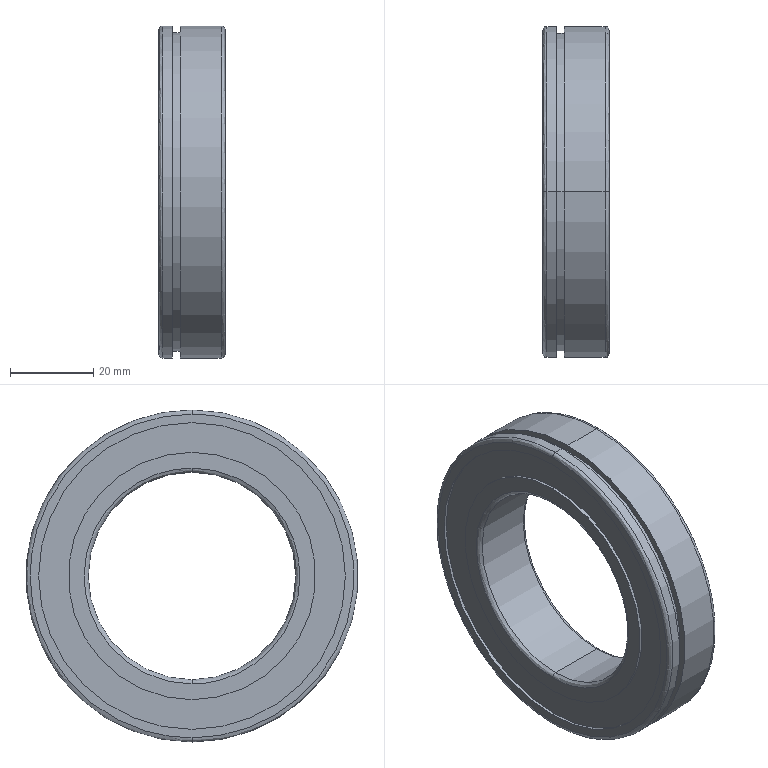Part | STEP file | 0229_Z_B6010ZZNR_1 | 1 solid | 32 faces | box 16 x 80 x 80 mm | volume 45982 mm3 | cylinder 16 | spline 8 | plane 8 | commonest cylinder face diameters 59.6 x4 73.92 x4 80 x4 50 x2 76.81 x2